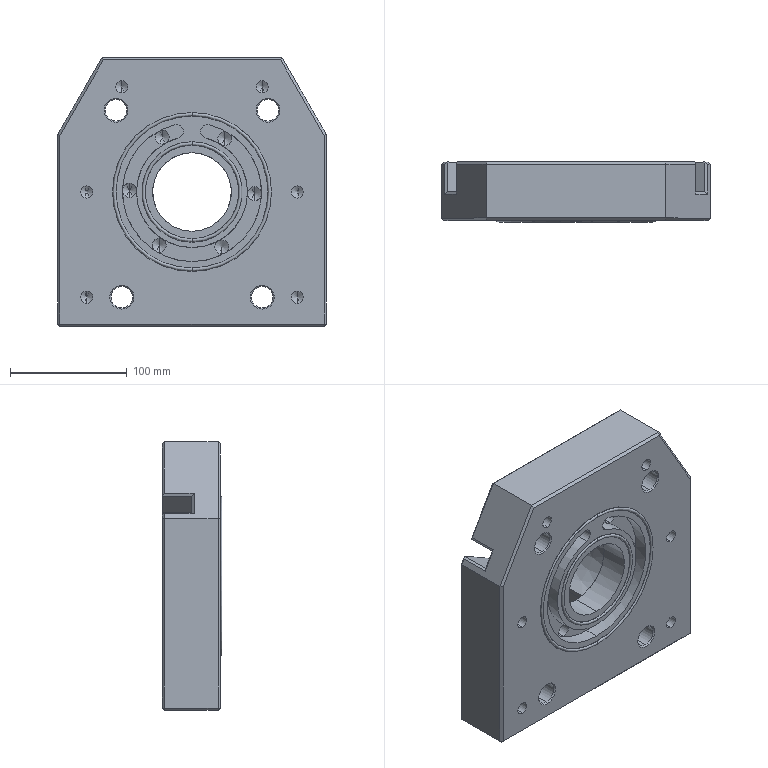Part | STEP file | Macho - Torre - 1 cav | 3 solids | 160 faces | box 230 x 51.25 x 230 mm | volume 2090171 mm3 | plane 66 | cylinder 50 | cone 36 | torus 8 | commonest cylinder face diameters 12 x16 10.5 x12 18.5 x8 67.284 x2 80 x2 86 x2